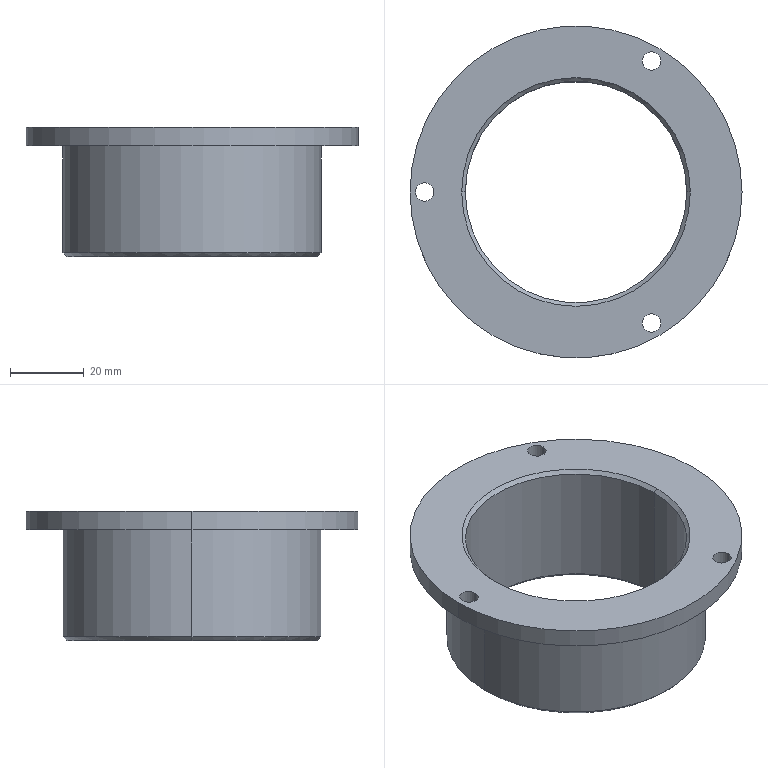Part | SolidWorks | features ICE 2, Chamfer 1, Extrusion 1 | 1 solid | 21 faces | box 90 x 90 x 35 mm | volume 47708 mm3 | cylinder 12 | cone 6 | plane 3 | commonest cylinder face diameters 5 x6 60 x2 70 x2 90 x2
STEP:
#1=CARTESIAN_POINT('',(-30.,0.,34.));
#2=VERTEX_POINT('',#1);
#3=CARTESIAN_POINT('',(30.,0.,34.));
#4=VERTEX_POINT('',#3);
#5=CARTESIAN_POINT('',(0.,0.,34.));
#6=DIRECTION('',(0.,0.,1.));
#7=DIRECTION('',(1.,0.,0.));
#8=AXIS2_PLACEMENT_3D('',#5,#6,#7);
#9=CIRCLE('',#8,30.);
#10=EDGE_CURVE('',#2,#4,#9,.T.);
#11=ORIENTED_EDGE('',*,*,#10,.F.);
#12=CARTESIAN_POINT('',(-31.,0.,35.));
#13=VERTEX_POINT('',#12);
#14=CARTESIAN_POINT('',(-30.,0.,34.));
#15=DIRECTION('',(-0.7071,0.,0.7071));
#16=VECTOR('',#15,1000.);
#17=LINE('',#14,#16);
#18=EDGE_CURVE('',#2,#13,#17,.T.);
#19=ORIENTED_EDGE('',*,*,#18,.T.);
#20=CARTESIAN_POINT('',(31.,0.,35.));
#21=VERTEX_POINT('',#20);
#22=CARTESIAN_POINT('',(0.,0.,35.));
#23=DIRECTION('',(0.,0.,-1.));
#24=DIRECTION('',(1.,0.,0.));
#25=AXIS2_PLACEMENT_3D('',#22,#23,#24);
#26=CIRCLE('',#25,31.);
#27=EDGE_CURVE('',#21,#13,#26,.T.);
#28=ORIENTED_EDGE('',*,*,#27,.F.);
#29=CARTESIAN_POINT('',(30.,0.,34.));
#30=DIRECTION('',(0.7071,0.,0.7071));
#31=VECTOR('',#30,1000.);
#32=LINE('',#29,#31);
#33=EDGE_CURVE('',#4,#21,#32,.T.);
#34=ORIENTED_EDGE('',*,*,#33,.F.);
#35=EDGE_LOOP('',(#11,#19,#28,#34));
#36=FACE_OUTER_BOUND('',#35,.T.);
#37=CARTESIAN_POINT('',(0.,0.,34.));
#38=DIRECTION('',(0.,0.,1.));
#39=DIRECTION('',(1.,0.,0.));
#40=AXIS2_PLACEMENT_3D('',#37,#38,#39);
#41=CONICAL_SURFACE('',#40,30.,0.7854);
#42=ADVANCED_FACE('',(#36),#41,.F.);
#43=CARTESIAN_POINT('',(-34.,0.,0.));
#44=VERTEX_POINT('',#43);
#45=CARTESIAN_POINT('',(34.,0.,0.));
#46=VERTEX_POINT('',#45);
#47=CARTESIAN_POINT('',(0.,0.,0.));
#48=DIRECTION('',(0.,0.,-1.));
#49=DIRECTION('',(1.,0.,0.));
#50=AXIS2_PLACEMENT_3D('',#47,#48,#49);
#51=CIRCLE('',#50,34.);
#52=EDGE_CURVE('',#44,#46,#51,.T.);
#53=ORIENTED_EDGE('',*,*,#52,.F.);
#54=CARTESIAN_POINT('',(-35.,0.,1.));
#55=VERTEX_POINT('',#54);
#56=CARTESIAN_POINT('',(-35.,0.,1.));
#57=DIRECTION('',(-0.7071,0.,0.7071));
#58=VECTOR('',#57,1000.);
#59=LINE('',#56,#58);
#60=EDGE_CURVE('',#44,#55,#59,.T.);
#61=ORIENTED_EDGE('',*,*,#60,.T.);
#62=CARTESIAN_POINT('',(35.,0.,1.));
#63=VERTEX_POINT('',#62);
#64=CARTESIAN_POINT('',(0.,0.,1.));
#65=DIRECTION('',(0.,0.,1.));
#66=DIRECTION('',(1.,0.,0.));
#67=AXIS2_PLACEMENT_3D('',#64,#65,#66);
#68=CIRCLE('',#67,35.);
#69=EDGE_CURVE('',#63,#55,#68,.T.);
#70=ORIENTED_EDGE('',*,*,#69,.F.);
#71=CARTESIAN_POINT('',(35.,0.,1.));
#72=DIRECTION('',(0.7071,0.,0.7071));
#73=VECTOR('',#72,1000.);
#74=LINE('',#71,#73);
#75=EDGE_CURVE('',#46,#63,#74,.T.);
#76=ORIENTED_EDGE('',*,*,#75,.F.);
#77=EDGE_LOOP('',(#53,#61,#70,#76));
#78=FACE_OUTER_BOUND('',#77,.T.);
#79=CARTESIAN_POINT('',(0.,0.,1.));
#80=DIRECTION('',(0.,0.,1.));
#81=DIRECTION('',(1.,0.,0.));
#82=AXIS2_PLACEMENT_3D('',#79,#80,#81);
#83=CONICAL_SURFACE('',#82,35.,0.7854);
#84=ADVANCED_FACE('',(#78),#83,.T.);
#85=CARTESIAN_POINT('',(30.,0.,1.));
#86=VERTEX_POINT('',#85);
#87=CARTESIAN_POINT('',(-30.,0.,1.));
#88=VERTEX_POINT('',#87);
#89=CARTESIAN_POINT('',(0.,0.,1.));
#90=DIRECTION('',(0.,0.,-1.));
#91=DIRECTION('',(1.,0.,0.));
#92=AXIS2_PLACEMENT_3D('',#89,#90,#91);
#93=CIRCLE('',#92,30.);
#94=EDGE_CURVE('',#86,#88,#93,.T.);
#95=ORIENTED_EDGE('',*,*,#94,.F.);
#96=CARTESIAN_POINT('',(31.,0.,0.));
#97=VERTEX_POINT('',#96);
#98=CARTESIAN_POINT('',(31.,0.,0.));
#99=DIRECTION('',(0.7071,0.,-0.7071));
#100=VECTOR('',#99,1000.);
#101=LINE('',#98,#100);
#102=EDGE_CURVE('',#86,#97,#101,.T.);
#103=ORIENTED_EDGE('',*,*,#102,.T.);
#104=CARTESIAN_POINT('',(-31.,0.,0.));
#105=VERTEX_POINT('',#104);
#106=CARTESIAN_POINT('',(0.,0.,0.));
#107=DIRECTION('',(0.,0.,1.));
#108=DIRECTION('',(1.,0.,0.));
#109=AXIS2_PLACEMENT_3D('',#106,#107,#108);
#110=CIRCLE('',#109,31.);
#111=EDGE_CURVE('',#105,#97,#110,.T.);
#112=ORIENTED_EDGE('',*,*,#111,.F.);
#113=CARTESIAN_POINT('',(-31.,0.,0.));
#114=DIRECTION('',(-0.7071,0.,-0.7071));
#115=VECTOR('',#114,1000.);
#116=LINE('',#113,#115);
#117=EDGE_CURVE('',#88,#105,#116,.T.);
#118=ORIENTED_EDGE('',*,*,#117,.F.);
#119=EDGE_LOOP('',(#95,#103,#112,#118));
#120=FACE_OUTER_BOUND('',#119,.T.);
#121=CARTESIAN_POINT('',(0.,0.,0.));
#122=DIRECTION('',(0.,0.,-1.));
#123=DIRECTION('',(-1.,0.,0.));
#124=AXIS2_PLACEMENT_3D('',#121,#122,#123);
#125=CONICAL_SURFACE('',#124,31.,0.7854);
#126=ADVANCED_FACE('',(#120),#125,.F.);
#127=CARTESIAN_POINT('',(-43.5,0.,35.));
#128=VERTEX_POINT('',#127);
#129=CARTESIAN_POINT('',(-38.5,0.,35.));
#130=VERTEX_POINT('',#129);
#131=CARTESIAN_POINT('',(-41.,0.,35.));
#132=DIRECTION('',(0.,0.,1.));
#133=DIRECTION('',(1.,0.,0.));
#134=AXIS2_PLACEMENT_3D('',#131,#132,#133);
#135=CIRCLE('',#134,2.5);
#136=EDGE_CURVE('',#128,#130,#135,.T.);
#137=ORIENTED_EDGE('',*,*,#136,.T.);
#138=CARTESIAN_POINT('',(-38.5,0.,30.));
#139=VERTEX_POINT('',#138);
#140=CARTESIAN_POINT('',(-38.5,0.,80.));
#141=DIRECTION('',(0.,0.,-1.));
#142=VECTOR('',#141,1000.);
#143=LINE('',#140,#142);
#144=EDGE_CURVE('',#130,#139,#143,.T.);
#145=ORIENTED_EDGE('',*,*,#144,.T.);
#146=CARTESIAN_POINT('',(-43.5,0.,30.));
#147=VERTEX_POINT('',#146);
#148=CARTESIAN_POINT('',(-41.,0.,30.));
#149=DIRECTION('',(0.,0.,-1.));
#150=DIRECTION('',(-1.,0.,0.));
#151=AXIS2_PLACEMENT_3D('',#148,#149,#150);
#152=CIRCLE('',#151,2.5);
#153=EDGE_CURVE('',#139,#147,#152,.T.);
#154=ORIENTED_EDGE('',*,*,#153,.T.);
#155=CARTESIAN_POINT('',(-43.5,0.,80.));
#156=DIRECTION('',(0.,0.,-1.));
#157=VECTOR('',#156,1000.);
#158=LINE('',#155,#157);
#159=EDGE_CURVE('',#128,#147,#158,.T.);
#160=ORIENTED_EDGE('',*,*,#159,.F.);
#161=EDGE_LOOP('',(#137,#145,#154,#160));
#162=FACE_OUTER_BOUND('',#161,.T.);
#163=CARTESIAN_POINT('',(-41.,0.,80.));
#164=DIRECTION('',(0.,0.,-1.));
#165=DIRECTION('',(-1.,0.,0.));
#166=AXIS2_PLACEMENT_3D('',#163,#164,#165);
#167=CYLINDRICAL_SURFACE('',#166,2.5);
#168=ADVANCED_FACE('',(#162),#167,.F.);
#169=CARTESIAN_POINT('',(18.,-35.507,35.));
#170=VERTEX_POINT('',#169);
#171=CARTESIAN_POINT('',(23.,-35.507,35.));
#172=VERTEX_POINT('',#171);
#173=CARTESIAN_POINT('',(20.5,-35.507,35.));
#174=DIRECTION('',(0.,0.,1.));
#175=DIRECTION('',(1.,0.,0.));
#176=AXIS2_PLACEMENT_3D('',#173,#174,#175);
#177=CIRCLE('',#176,2.5);
#178=EDGE_CURVE('',#170,#172,#177,.T.);
#179=ORIENTED_EDGE('',*,*,#178,.T.);
#180=CARTESIAN_POINT('',(23.,-35.507,30.));
#181=VERTEX_POINT('',#180);
#182=CARTESIAN_POINT('',(23.,-35.507,80.));
#183=DIRECTION('',(0.,0.,-1.));
#184=VECTOR('',#183,1000.);
#185=LINE('',#182,#184);
#186=EDGE_CURVE('',#172,#181,#185,.T.);
#187=ORIENTED_EDGE('',*,*,#186,.T.);
#188=CARTESIAN_POINT('',(18.,-35.507,30.));
#189=VERTEX_POINT('',#188);
#190=CARTESIAN_POINT('',(20.5,-35.507,30.));
#191=DIRECTION('',(0.,0.,-1.));
#192=DIRECTION('',(-1.,0.,0.));
#193=AXIS2_PLACEMENT_3D('',#190,#191,#192);
#194=CIRCLE('',#193,2.5);
#195=EDGE_CURVE('',#181,#189,#194,.T.);
#196=ORIENTED_EDGE('',*,*,#195,.T.);
#197=CARTESIAN_POINT('',(18.,-35.507,80.));
#198=DIRECTION('',(0.,0.,-1.));
#199=VECTOR('',#198,1000.);
#200=LINE('',#197,#199);
#201=EDGE_CURVE('',#170,#189,#200,.T.);
#202=ORIENTED_EDGE('',*,*,#201,.F.);
#203=EDGE_LOOP('',(#179,#187,#196,#202));
#204=FACE_OUTER_BOUND('',#203,.T.);
#205=CARTESIAN_POINT('',(20.5,-35.507,80.));
#206=DIRECTION('',(0.,0.,-1.));
#207=DIRECTION('',(-1.,0.,0.));
#208=AXIS2_PLACEMENT_3D('',#205,#206,#207);
#209=CYLINDRICAL_SURFACE('',#208,2.5);
#210=ADVANCED_FACE('',(#204),#209,.F.);
#211=CARTESIAN_POINT('',(18.,35.507,35.));
#212=VERTEX_POINT('',#211);
#213=CARTESIAN_POINT('',(23.,35.507,35.));
#214=VERTEX_POINT('',#213);
#215=CARTESIAN_POINT('',(20.5,35.507,35.));
#216=DIRECTION('',(0.,0.,1.));
#217=DIRECTION('',(1.,0.,0.));
#218=AXIS2_PLACEMENT_3D('',#215,#216,#217);
#219=CIRCLE('',#218,2.5);
#220=EDGE_CURVE('',#212,#214,#219,.T.);
#221=ORIENTED_EDGE('',*,*,#220,.T.);
#222=CARTESIAN_POINT('',(23.,35.507,30.));
#223=VERTEX_POINT('',#222);
#224=CARTESIAN_POINT('',(23.,35.507,80.));
#225=DIRECTION('',(0.,0.,-1.));
#226=VECTOR('',#225,1000.);
#227=LINE('',#224,#226);
#228=EDGE_CURVE('',#214,#223,#227,.T.);
#229=ORIENTED_EDGE('',*,*,#228,.T.);
#230=CARTESIAN_POINT('',(18.,35.507,30.));
#231=VERTEX_POINT('',#230);
#232=CARTESIAN_POINT('',(20.5,35.507,30.));
#233=DIRECTION('',(0.,0.,-1.));
#234=DIRECTION('',(-1.,0.,0.));
#235=AXIS2_PLACEMENT_3D('',#232,#233,#234);
#236=CIRCLE('',#235,2.5);
#237=EDGE_CURVE('',#223,#231,#236,.T.);
#238=ORIENTED_EDGE('',*,*,#237,.T.);
#239=CARTESIAN_POINT('',(18.,35.507,80.));
#240=DIRECTION('',(0.,0.,-1.));
#241=VECTOR('',#240,1000.);
#242=LINE('',#239,#241);
#243=EDGE_CURVE('',#212,#231,#242,.T.);
#244=ORIENTED_EDGE('',*,*,#243,.F.);
#245=EDGE_LOOP('',(#221,#229,#238,#244));
#246=FACE_OUTER_BOUND('',#245,.T.);
#247=CARTESIAN_POINT('',(20.5,35.507,80.));
#248=DIRECTION('',(0.,0.,-1.));
#249=DIRECTION('',(-1.,0.,0.));
#250=AXIS2_PLACEMENT_3D('',#247,#248,#249);
#251=CYLINDRICAL_SURFACE('',#250,2.5);
#252=ADVANCED_FACE('',(#246),#251,.F.);
#253=CARTESIAN_POINT('',(45.,0.,35.));
#254=VERTEX_POINT('',#253);
#255=CARTESIAN_POINT('',(-45.,0.,35.));
#256=VERTEX_POINT('',#255);
#257=CARTESIAN_POINT('',(0.,0.,35.));
#258=DIRECTION('',(0.,0.,1.));
#259=DIRECTION('',(1.,0.,0.));
#260=AXIS2_PLACEMENT_3D('',#257,#258,#259);
#261=CIRCLE('',#260,45.);
#262=EDGE_CURVE('',#254,#256,#261,.T.);
#263=ORIENTED_EDGE('',*,*,#262,.F.);
#264=CARTESIAN_POINT('',(45.,0.,30.));
#265=VERTEX_POINT('',#264);
#266=CARTESIAN_POINT('',(45.,0.,35.));
#267=DIRECTION('',(0.,0.,-1.));
#268=VECTOR('',#267,1000.);
#269=LINE('',#266,#268);
#270=EDGE_CURVE('',#254,#265,#269,.T.);
#271=ORIENTED_EDGE('',*,*,#270,.T.);
#272=CARTESIAN_POINT('',(-45.,0.,30.));
#273=VERTEX_POINT('',#272);
#274=CARTESIAN_POINT('',(0.,0.,30.));
#275=DIRECTION('',(0.,0.,1.));
#276=DIRECTION('',(1.,0.,0.));
#277=AXIS2_PLACEMENT_3D('',#274,#275,#276);
#278=CIRCLE('',#277,45.);
#279=EDGE_CURVE('',#265,#273,#278,.T.);
#280=ORIENTED_EDGE('',*,*,#279,.T.);
#281=CARTESIAN_POINT('',(-45.,0.,35.));
#282=DIRECTION('',(0.,0.,-1.));
#283=VECTOR('',#282,1000.);
#284=LINE('',#281,#283);
#285=EDGE_CURVE('',#256,#273,#284,.T.);
#286=ORIENTED_EDGE('',*,*,#285,.F.);
#287=EDGE_LOOP('',(#263,#271,#280,#286));
#288=FACE_OUTER_BOUND('',#287,.T.);
#289=CARTESIAN_POINT('',(0.,0.,35.));
#290=DIRECTION('',(0.,0.,-1.));
#291=DIRECTION('',(-1.,0.,0.));
#292=AXIS2_PLACEMENT_3D('',#289,#290,#291);
#293=CYLINDRICAL_SURFACE('',#292,45.);
#294=ADVANCED_FACE('',(#288),#293,.T.);
#295=ORIENTED_EDGE('',*,*,#10,.T.);
#296=CARTESIAN_POINT('',(30.,0.,30.));
#297=DIRECTION('',(0.,0.,-1.));
#298=VECTOR('',#297,1000.);
#299=LINE('',#296,#298);
#300=EDGE_CURVE('',#4,#86,#299,.T.);
#301=ORIENTED_EDGE('',*,*,#300,.T.);
#302=ORIENTED_EDGE('',*,*,#94,.T.);
#303=CARTESIAN_POINT('',(-30.,0.,30.));
#304=DIRECTION('',(0.,0.,-1.));
#305=VECTOR('',#304,1000.);
#306=LINE('',#303,#305);
#307=EDGE_CURVE('',#2,#88,#306,.T.);
#308=ORIENTED_EDGE('',*,*,#307,.F.);
#309=EDGE_LOOP('',(#295,#301,#302,#308));
#310=FACE_OUTER_BOUND('',#309,.T.);
#311=CARTESIAN_POINT('',(0.,0.,30.));
#312=DIRECTION('',(0.,0.,-1.));
#313=DIRECTION('',(-1.,0.,0.));
#314=AXIS2_PLACEMENT_3D('',#311,#312,#313);
#315=CYLINDRICAL_SURFACE('',#314,30.);
#316=ADVANCED_FACE('',(#310),#315,.F.);
#317=CARTESIAN_POINT('',(35.,0.,30.));
#318=VERTEX_POINT('',#317);
#319=CARTESIAN_POINT('',(-35.,0.,30.));
#320=VERTEX_POINT('',#319);
#321=CARTESIAN_POINT('',(0.,0.,30.));
#322=DIRECTION('',(0.,0.,1.));
#323=DIRECTION('',(1.,0.,0.));
#324=AXIS2_PLACEMENT_3D('',#321,#322,#323);
#325=CIRCLE('',#324,35.);
#326=EDGE_CURVE('',#318,#320,#325,.T.);
#327=ORIENTED_EDGE('',*,*,#326,.F.);
#328=CARTESIAN_POINT('',(35.,0.,30.));
#329=DIRECTION('',(0.,0.,-1.));
#330=VECTOR('',#329,1000.);
#331=LINE('',#328,#330);
#332=EDGE_CURVE('',#318,#63,#331,.T.);
#333=ORIENTED_EDGE('',*,*,#332,.T.);
#334=ORIENTED_EDGE('',*,*,#69,.T.);
#335=CARTESIAN_POINT('',(-35.,0.,30.));
#336=DIRECTION('',(0.,0.,-1.));
#337=VECTOR('',#336,1000.);
#338=LINE('',#335,#337);
#339=EDGE_CURVE('',#320,#55,#338,.T.);
#340=ORIENTED_EDGE('',*,*,#339,.F.);
#341=EDGE_LOOP('',(#327,#333,#334,#340));
#342=FACE_OUTER_BOUND('',#341,.T.);
#343=CARTESIAN_POINT('',(0.,0.,30.));
#344=DIRECTION('',(0.,0.,-1.));
#345=DIRECTION('',(-1.,0.,0.));
#346=AXIS2_PLACEMENT_3D('',#343,#344,#345);
#347=CYLINDRICAL_SURFACE('',#346,35.);
#348=ADVANCED_FACE('',(#342),#347,.T.);
#349=ORIENTED_EDGE('',*,*,#111,.T.);
#350=CARTESIAN_POINT('',(0.,0.,0.));
#351=DIRECTION('',(0.,0.,1.));
#352=DIRECTION('',(1.,0.,0.));
#353=AXIS2_PLACEMENT_3D('',#350,#351,#352);
#354=CIRCLE('',#353,31.);
#355=EDGE_CURVE('',#97,#105,#354,.T.);
#356=ORIENTED_EDGE('',*,*,#355,.T.);
#357=EDGE_LOOP('',(#349,#356));
#358=FACE_BOUND('',#357,.T.);
#359=CARTESIAN_POINT('',(0.,0.,0.));
#360=DIRECTION('',(0.,0.,-1.));
#361=DIRECTION('',(1.,0.,0.));
#362=AXIS2_PLACEMENT_3D('',#359,#360,#361);
#363=CIRCLE('',#362,34.);
#364=EDGE_CURVE('',#46,#44,#363,.T.);
#365=ORIENTED_EDGE('',*,*,#364,.T.);
#366=ORIENTED_EDGE('',*,*,#52,.T.);
#367=EDGE_LOOP('',(#365,#366));
#368=FACE_OUTER_BOUND('',#367,.T.);
#369=CARTESIAN_POINT('',(0.,0.,0.));
#370=DIRECTION('',(0.,0.,1.));
#371=DIRECTION('',(1.,0.,0.));
#372=AXIS2_PLACEMENT_3D('',#369,#370,#371);
#373=PLANE('',#372);
#374=ADVANCED_FACE('',(#358,#368),#373,.F.);
#375=ORIENTED_EDGE('',*,*,#332,.F.);
#376=CARTESIAN_POINT('',(0.,0.,30.));
#377=DIRECTION('',(0.,0.,1.));
#378=DIRECTION('',(1.,0.,0.));
#379=AXIS2_PLACEMENT_3D('',#376,#377,#378);
#380=CIRCLE('',#379,35.);
#381=EDGE_CURVE('',#320,#318,#380,.T.);
#382=ORIENTED_EDGE('',*,*,#381,.F.);
#383=ORIENTED_EDGE('',*,*,#339,.T.);
#384=CARTESIAN_POINT('',(0.,0.,1.));
#385=DIRECTION('',(0.,0.,1.));
#386=DIRECTION('',(1.,0.,0.));
#387=AXIS2_PLACEMENT_3D('',#384,#385,#386);
#388=CIRCLE('',#387,35.);
#389=EDGE_CURVE('',#55,#63,#388,.T.);
#390=ORIENTED_EDGE('',*,*,#389,.T.);
#391=EDGE_LOOP('',(#375,#382,#383,#390));
#392=FACE_OUTER_BOUND('',#391,.T.);
#393=CARTESIAN_POINT('',(0.,0.,30.));
#394=DIRECTION('',(0.,0.,-1.));
#395=DIRECTION('',(-1.,0.,0.));
#396=AXIS2_PLACEMENT_3D('',#393,#394,#395);
#397=CYLINDRICAL_SURFACE('',#396,35.);
#398=ADVANCED_FACE('',(#392),#397,.T.);
#399=ORIENTED_EDGE('',*,*,#300,.F.);
#400=CARTESIAN_POINT('',(0.,0.,34.));
#401=DIRECTION('',(0.,0.,1.));
#402=DIRECTION('',(1.,0.,0.));
#403=AXIS2_PLACEMENT_3D('',#400,#401,#402);
#404=CIRCLE('',#403,30.);
#405=EDGE_CURVE('',#4,#2,#404,.T.);
#406=ORIENTED_EDGE('',*,*,#405,.T.);
#407=ORIENTED_EDGE('',*,*,#307,.T.);
#408=CARTESIAN_POINT('',(0.,0.,1.));
#409=DIRECTION('',(0.,0.,-1.));
#410=DIRECTION('',(1.,0.,0.));
#411=AXIS2_PLACEMENT_3D('',#408,#409,#410);
#412=CIRCLE('',#411,30.);
#413=EDGE_CURVE('',#88,#86,#412,.T.);
#414=ORIENTED_EDGE('',*,*,#413,.T.);
#415=EDGE_LOOP('',(#399,#406,#407,#414));
#416=FACE_OUTER_BOUND('',#415,.T.);
#417=CARTESIAN_POINT('',(0.,0.,30.));
#418=DIRECTION('',(0.,0.,-1.));
#419=DIRECTION('',(-1.,0.,0.));
#420=AXIS2_PLACEMENT_3D('',#417,#418,#419);
#421=CYLINDRICAL_SURFACE('',#420,30.);
#422=ADVANCED_FACE('',(#416),#421,.F.);
#423=ORIENTED_EDGE('',*,*,#27,.T.);
#424=CARTESIAN_POINT('',(0.,0.,35.));
#425=DIRECTION('',(0.,0.,-1.));
#426=DIRECTION('',(1.,0.,0.));
#427=AXIS2_PLACEMENT_3D('',#424,#425,#426);
#428=CIRCLE('',#427,31.);
#429=EDGE_CURVE('',#13,#21,#428,.T.);
#430=ORIENTED_EDGE('',*,*,#429,.T.);
#431=EDGE_LOOP('',(#423,#430));
#432=FACE_BOUND('',#431,.T.);
#433=ORIENTED_EDGE('',*,*,#136,.F.);
#434=CARTESIAN_POINT('',(-41.,0.,35.));
#435=DIRECTION('',(0.,0.,1.));
#436=DIRECTION('',(1.,0.,0.));
#437=AXIS2_PLACEMENT_3D('',#434,#435,#436);
#438=CIRCLE('',#437,2.5);
#439=EDGE_CURVE('',#130,#128,#438,.T.);
#440=ORIENTED_EDGE('',*,*,#439,.F.);
#441=EDGE_LOOP('',(#433,#440));
#442=FACE_BOUND('',#441,.T.);
#443=ORIENTED_EDGE('',*,*,#178,.F.);
#444=CARTESIAN_POINT('',(20.5,-35.507,35.));
#445=DIRECTION('',(0.,0.,1.));
#446=DIRECTION('',(1.,0.,0.));
#447=AXIS2_PLACEMENT_3D('',#444,#445,#446);
#448=CIRCLE('',#447,2.5);
#449=EDGE_CURVE('',#172,#170,#448,.T.);
#450=ORIENTED_EDGE('',*,*,#449,.F.);
#451=EDGE_LOOP('',(#443,#450));
#452=FACE_BOUND('',#451,.T.);
#453=ORIENTED_EDGE('',*,*,#220,.F.);
#454=CARTESIAN_POINT('',(20.5,35.507,35.));
#455=DIRECTION('',(0.,0.,1.));
#456=DIRECTION('',(1.,0.,0.));
#457=AXIS2_PLACEMENT_3D('',#454,#455,#456);
#458=CIRCLE('',#457,2.5);
#459=EDGE_CURVE('',#214,#212,#458,.T.);
#460=ORIENTED_EDGE('',*,*,#459,.F.);
#461=EDGE_LOOP('',(#453,#460));
#462=FACE_BOUND('',#461,.T.);
#463=CARTESIAN_POINT('',(0.,0.,35.));
#464=DIRECTION('',(0.,0.,1.));
#465=DIRECTION('',(1.,0.,0.));
#466=AXIS2_PLACEMENT_3D('',#463,#464,#465);
#467=CIRCLE('',#466,45.);
#468=EDGE_CURVE('',#256,#254,#467,.T.);
#469=ORIENTED_EDGE('',*,*,#468,.T.);
#470=ORIENTED_EDGE('',*,*,#262,.T.);
#471=EDGE_LOOP('',(#469,#470));
#472=FACE_OUTER_BOUND('',#471,.T.);
#473=CARTESIAN_POINT('',(0.,0.,35.));
#474=DIRECTION('',(0.,0.,1.));
#475=DIRECTION('',(1.,0.,0.));
#476=AXIS2_PLACEMENT_3D('',#473,#474,#475);
#477=PLANE('',#476);
#478=ADVANCED_FACE('',(#432,#442,#452,#462,#472),#477,.T.);
#479=CARTESIAN_POINT('',(-41.,0.,30.));
#480=DIRECTION('',(0.,0.,-1.));
#481=DIRECTION('',(-1.,0.,0.));
#482=AXIS2_PLACEMENT_3D('',#479,#480,#481);
#483=CIRCLE('',#482,2.5);
#484=EDGE_CURVE('',#147,#139,#483,.T.);
#485=ORIENTED_EDGE('',*,*,#484,.F.);
#486=ORIENTED_EDGE('',*,*,#153,.F.);
#487=EDGE_LOOP('',(#485,#486));
#488=FACE_BOUND('',#487,.T.);
#489=CARTESIAN_POINT('',(20.5,-35.507,30.));
#490=DIRECTION('',(0.,0.,-1.));
#491=DIRECTION('',(-1.,0.,0.));
#492=AXIS2_PLACEMENT_3D('',#489,#490,#491);
#493=CIRCLE('',#492,2.5);
#494=EDGE_CURVE('',#189,#181,#493,.T.);
#495=ORIENTED_EDGE('',*,*,#494,.F.);
#496=ORIENTED_EDGE('',*,*,#195,.F.);
#497=EDGE_LOOP('',(#495,#496));
#498=FACE_BOUND('',#497,.T.);
#499=CARTESIAN_POINT('',(20.5,35.507,30.));
#500=DIRECTION('',(0.,0.,-1.));
#501=DIRECTION('',(-1.,0.,0.));
#502=AXIS2_PLACEMENT_3D('',#499,#500,#501);
#503=CIRCLE('',#502,2.5);
#504=EDGE_CURVE('',#231,#223,#503,.T.);
#505=ORIENTED_EDGE('',*,*,#504,.F.);
#506=ORIENTED_EDGE('',*,*,#237,.F.);
#507=EDGE_LOOP('',(#505,#506));
#508=FACE_BOUND('',#507,.T.);
#509=ORIENTED_EDGE('',*,*,#381,.T.);
#510=ORIENTED_EDGE('',*,*,#326,.T.);
#511=EDGE_LOOP('',(#509,#510));
#512=FACE_BOUND('',#511,.T.);
#513=CARTESIAN_POINT('',(0.,0.,30.));
#514=DIRECTION('',(0.,0.,1.));
#515=DIRECTION('',(1.,0.,0.));
#516=AXIS2_PLACEMENT_3D('',#513,#514,#515);
#517=CIRCLE('',#516,45.);
#518=EDGE_CURVE('',#273,#265,#517,.T.);
#519=ORIENTED_EDGE('',*,*,#518,.F.);
#520=ORIENTED_EDGE('',*,*,#279,.F.);
#521=EDGE_LOOP('',(#519,#520));
#522=FACE_OUTER_BOUND('',#521,.T.);
#523=CARTESIAN_POINT('',(0.,0.,30.));
#524=DIRECTION('',(0.,0.,1.));
#525=DIRECTION('',(1.,0.,0.));
#526=AXIS2_PLACEMENT_3D('',#523,#524,#525);
#527=PLANE('',#526);
#528=ADVANCED_FACE('',(#488,#498,#508,#512,#522),#527,.F.);
#529=ORIENTED_EDGE('',*,*,#270,.F.);
#530=ORIENTED_EDGE('',*,*,#468,.F.);
#531=ORIENTED_EDGE('',*,*,#285,.T.);
#532=ORIENTED_EDGE('',*,*,#518,.T.);
#533=EDGE_LOOP('',(#529,#530,#531,#532));
#534=FACE_OUTER_BOUND('',#533,.T.);
#535=CARTESIAN_POINT('',(0.,0.,35.));
#536=DIRECTION('',(0.,0.,-1.));
#537=DIRECTION('',(-1.,0.,0.));
#538=AXIS2_PLACEMENT_3D('',#535,#536,#537);
#539=CYLINDRICAL_SURFACE('',#538,45.);
#540=ADVANCED_FACE('',(#534),#539,.T.);
#541=ORIENTED_EDGE('',*,*,#228,.F.);
#542=ORIENTED_EDGE('',*,*,#459,.T.);
#543=ORIENTED_EDGE('',*,*,#243,.T.);
#544=ORIENTED_EDGE('',*,*,#504,.T.);
#545=EDGE_LOOP('',(#541,#542,#543,#544));
#546=FACE_OUTER_BOUND('',#545,.T.);
#547=CARTESIAN_POINT('',(20.5,35.507,80.));
#548=DIRECTION('',(0.,0.,-1.));
#549=DIRECTION('',(-1.,0.,0.));
#550=AXIS2_PLACEMENT_3D('',#547,#548,#549);
#551=CYLINDRICAL_SURFACE('',#550,2.5);
#552=ADVANCED_FACE('',(#546),#551,.F.);
#553=ORIENTED_EDGE('',*,*,#186,.F.);
#554=ORIENTED_EDGE('',*,*,#449,.T.);
#555=ORIENTED_EDGE('',*,*,#201,.T.);
#556=ORIENTED_EDGE('',*,*,#494,.T.);
#557=EDGE_LOOP('',(#553,#554,#555,#556));
#558=FACE_OUTER_BOUND('',#557,.T.);
#559=CARTESIAN_POINT('',(20.5,-35.507,80.));
#560=DIRECTION('',(0.,0.,-1.));
#561=DIRECTION('',(-1.,0.,0.));
#562=AXIS2_PLACEMENT_3D('',#559,#560,#561);
#563=CYLINDRICAL_SURFACE('',#562,2.5);
#564=ADVANCED_FACE('',(#558),#563,.F.);
#565=ORIENTED_EDGE('',*,*,#144,.F.);
#566=ORIENTED_EDGE('',*,*,#439,.T.);
#567=ORIENTED_EDGE('',*,*,#159,.T.);
#568=ORIENTED_EDGE('',*,*,#484,.T.);
#569=EDGE_LOOP('',(#565,#566,#567,#568));
#570=FACE_OUTER_BOUND('',#569,.T.);
#571=CARTESIAN_POINT('',(-41.,0.,80.));
#572=DIRECTION('',(0.,0.,-1.));
#573=DIRECTION('',(-1.,0.,0.));
#574=AXIS2_PLACEMENT_3D('',#571,#572,#573);
#575=CYLINDRICAL_SURFACE('',#574,2.5);
#576=ADVANCED_FACE('',(#570),#575,.F.);
#577=ORIENTED_EDGE('',*,*,#102,.F.);
#578=ORIENTED_EDGE('',*,*,#413,.F.);
#579=ORIENTED_EDGE('',*,*,#117,.T.);
#580=ORIENTED_EDGE('',*,*,#355,.F.);
#581=EDGE_LOOP('',(#577,#578,#579,#580));
#582=FACE_OUTER_BOUND('',#581,.T.);
#583=CARTESIAN_POINT('',(0.,0.,0.));
#584=DIRECTION('',(0.,0.,-1.));
#585=DIRECTION('',(-1.,0.,0.));
#586=AXIS2_PLACEMENT_3D('',#583,#584,#585);
#587=CONICAL_SURFACE('',#586,31.,0.7854);
#588=ADVANCED_FACE('',(#582),#587,.F.);
#589=ORIENTED_EDGE('',*,*,#60,.F.);
#590=ORIENTED_EDGE('',*,*,#364,.F.);
#591=ORIENTED_EDGE('',*,*,#75,.T.);
#592=ORIENTED_EDGE('',*,*,#389,.F.);
#593=EDGE_LOOP('',(#589,#590,#591,#592));
#594=FACE_OUTER_BOUND('',#593,.T.);
#595=CARTESIAN_POINT('',(0.,0.,1.));
#596=DIRECTION('',(0.,0.,1.));
#597=DIRECTION('',(1.,0.,0.));
#598=AXIS2_PLACEMENT_3D('',#595,#596,#597);
#599=CONICAL_SURFACE('',#598,35.,0.7854);
#600=ADVANCED_FACE('',(#594),#599,.T.);
#601=ORIENTED_EDGE('',*,*,#18,.F.);
#602=ORIENTED_EDGE('',*,*,#405,.F.);
#603=ORIENTED_EDGE('',*,*,#33,.T.);
#604=ORIENTED_EDGE('',*,*,#429,.F.);
#605=EDGE_LOOP('',(#601,#602,#603,#604));
#606=FACE_OUTER_BOUND('',#605,.T.);
#607=CARTESIAN_POINT('',(0.,0.,34.));
#608=DIRECTION('',(0.,0.,1.));
#609=DIRECTION('',(1.,0.,0.));
#610=AXIS2_PLACEMENT_3D('',#607,#608,#609);
#611=CONICAL_SURFACE('',#610,30.,0.7854);
#612=ADVANCED_FACE('',(#606),#611,.F.);
#613=CLOSED_SHELL('',(#42,#84,#126,#168,#210,#252,#294,#316,#348,#374,#398,#422,#478,#528,#540,#552,#564,#576,#588,#600,#612));
#614=MANIFOLD_SOLID_BREP('',#613);
#615=CARTESIAN_POINT('',(0.,0.,0.));
#616=DIRECTION('',(0.,0.,1.));
#617=DIRECTION('',(1.,0.,0.));
#618=AXIS2_PLACEMENT_3D('',#615,#616,#617);
#619=(LENGTH_UNIT()NAMED_UNIT(*)SI_UNIT(.MILLI.,.METRE.));
#620=UNCERTAINTY_MEASURE_WITH_UNIT(LENGTH_MEASURE(0.00001),#619,'','');
#621=(NAMED_UNIT(*)PLANE_ANGLE_UNIT()SI_UNIT($,.RADIAN.));
#622=(NAMED_UNIT(*)SI_UNIT($,.STERADIAN.)SOLID_ANGLE_UNIT());
#623=(GEOMETRIC_REPRESENTATION_CONTEXT(3)GLOBAL_UNCERTAINTY_ASSIGNED_CONTEXT((#620))GLOBAL_UNIT_ASSIGNED_CONTEXT((#619,#621,#622))REPRESENTATION_CONTEXT('',''));
#624=ADVANCED_BREP_SHAPE_REPRESENTATION('',(#614,#618),#623);